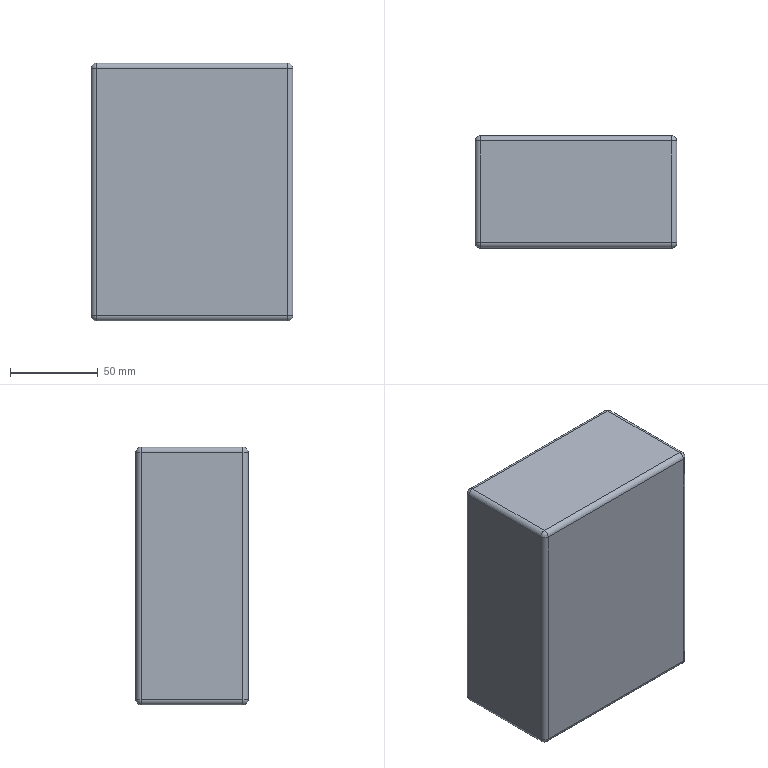Part | STEP file | PRODUCT_ID_95 | 1 solid | 26 faces | box 115 x 64 x 147 mm | volume 1079438 mm3 | cylinder 12 | sphere 8 | plane 6 | commonest cylinder face diameters 6 x12